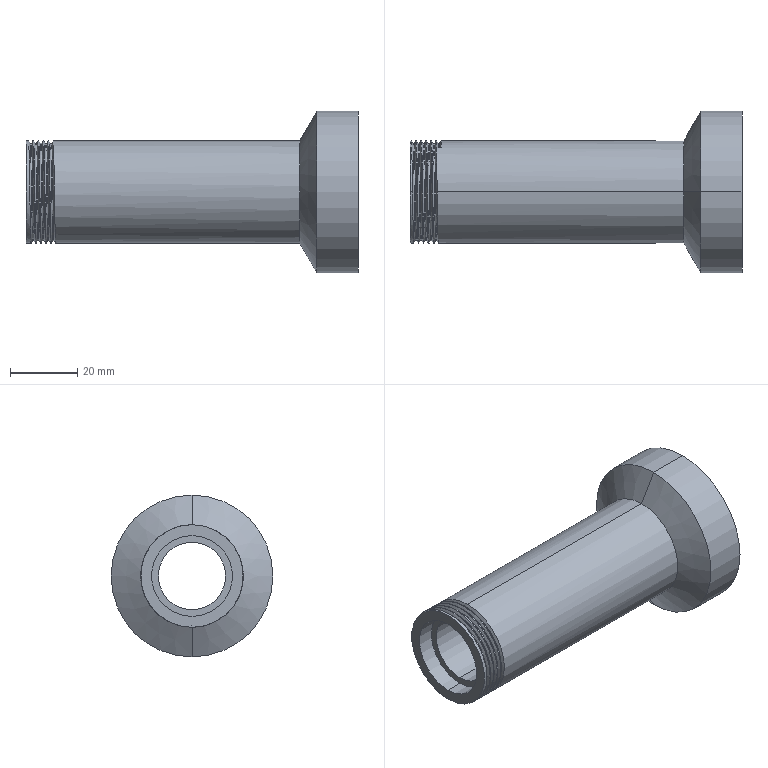Part | SolidWorks | features ICE 2, SweepThread 2, Revolution 1 | 1 solid | 48 faces | box 98.457 x 48 x 48 mm | volume 45862 mm3 | cylinder 30 | plane 8 | spline 6 | cone 4 | commonest cylinder face diameters 30.444 x12 36 x12 20 x2 24 x2 48 x2